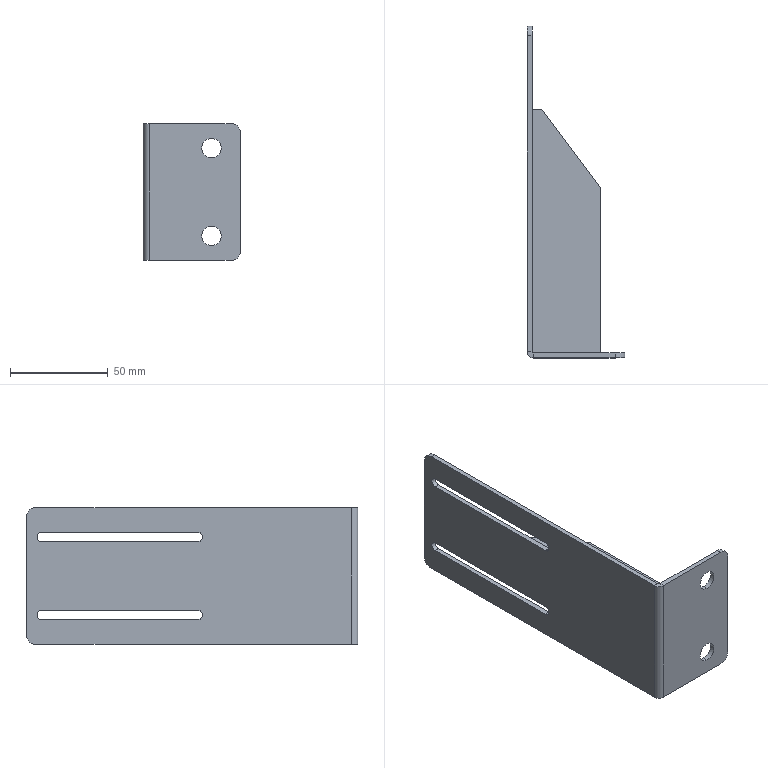Part | SolidWorks | features HoleWzd 2, BreakCorner 1, FlatPattern 1, Gusset 1, SMBaseFlange 1, SheetMetal 1 | 2 solids | 37 faces | box 50 x 170 x 70 mm | volume 44894 mm3 | plane 23 | cylinder 14 | commonest cylinder face diameters 10 x8 4.8 x4 1.473 x1 6.473 x1
STEP:
#1=CARTESIAN_POINT('',(35.,0.,7.5));
#2=VERTEX_POINT('',#1);
#3=CARTESIAN_POINT('',(35.,0.,17.5));
#4=VERTEX_POINT('',#3);
#5=CARTESIAN_POINT('',(35.,0.,12.5));
#6=DIRECTION('',(0.,1.,0.));
#7=DIRECTION('',(0.,0.,1.));
#8=AXIS2_PLACEMENT_3D('',#5,#6,#7);
#9=CIRCLE('',#8,5.);
#10=EDGE_CURVE('',#2,#4,#9,.T.);
#11=ORIENTED_EDGE('',*,*,#10,.F.);
#12=CARTESIAN_POINT('',(35.,2.5,7.5));
#13=VERTEX_POINT('',#12);
#14=CARTESIAN_POINT('',(35.,2.5,7.5));
#15=DIRECTION('',(0.,1.,0.));
#16=VECTOR('',#15,1000.);
#17=LINE('',#14,#16);
#18=EDGE_CURVE('',#2,#13,#17,.T.);
#19=ORIENTED_EDGE('',*,*,#18,.T.);
#20=CARTESIAN_POINT('',(35.,2.5,17.5));
#21=VERTEX_POINT('',#20);
#22=CARTESIAN_POINT('',(35.,2.5,12.5));
#23=DIRECTION('',(0.,1.,0.));
#24=DIRECTION('',(0.,0.,1.));
#25=AXIS2_PLACEMENT_3D('',#22,#23,#24);
#26=CIRCLE('',#25,5.);
#27=EDGE_CURVE('',#13,#21,#26,.T.);
#28=ORIENTED_EDGE('',*,*,#27,.T.);
#29=CARTESIAN_POINT('',(35.,2.5,17.5));
#30=DIRECTION('',(0.,1.,0.));
#31=VECTOR('',#30,1000.);
#32=LINE('',#29,#31);
#33=EDGE_CURVE('',#4,#21,#32,.T.);
#34=ORIENTED_EDGE('',*,*,#33,.F.);
#35=EDGE_LOOP('',(#11,#19,#28,#34));
#36=FACE_OUTER_BOUND('',#35,.T.);
#37=CARTESIAN_POINT('',(35.,2.5,12.5));
#38=DIRECTION('',(0.,1.,0.));
#39=DIRECTION('',(0.,0.,1.));
#40=AXIS2_PLACEMENT_3D('',#37,#38,#39);
#41=CYLINDRICAL_SURFACE('',#40,5.);
#42=ADVANCED_FACE('',(#36),#41,.F.);
#43=CARTESIAN_POINT('',(35.,0.,52.5));
#44=VERTEX_POINT('',#43);
#45=CARTESIAN_POINT('',(35.,0.,62.5));
#46=VERTEX_POINT('',#45);
#47=CARTESIAN_POINT('',(35.,0.,57.5));
#48=DIRECTION('',(0.,1.,0.));
#49=DIRECTION('',(0.,0.,1.));
#50=AXIS2_PLACEMENT_3D('',#47,#48,#49);
#51=CIRCLE('',#50,5.);
#52=EDGE_CURVE('',#44,#46,#51,.T.);
#53=ORIENTED_EDGE('',*,*,#52,.F.);
#54=CARTESIAN_POINT('',(35.,2.5,52.5));
#55=VERTEX_POINT('',#54);
#56=CARTESIAN_POINT('',(35.,2.5,52.5));
#57=DIRECTION('',(0.,1.,0.));
#58=VECTOR('',#57,1000.);
#59=LINE('',#56,#58);
#60=EDGE_CURVE('',#44,#55,#59,.T.);
#61=ORIENTED_EDGE('',*,*,#60,.T.);
#62=CARTESIAN_POINT('',(35.,2.5,62.5));
#63=VERTEX_POINT('',#62);
#64=CARTESIAN_POINT('',(35.,2.5,57.5));
#65=DIRECTION('',(0.,1.,0.));
#66=DIRECTION('',(0.,0.,1.));
#67=AXIS2_PLACEMENT_3D('',#64,#65,#66);
#68=CIRCLE('',#67,5.);
#69=EDGE_CURVE('',#55,#63,#68,.T.);
#70=ORIENTED_EDGE('',*,*,#69,.T.);
#71=CARTESIAN_POINT('',(35.,2.5,62.5));
#72=DIRECTION('',(0.,1.,0.));
#73=VECTOR('',#72,1000.);
#74=LINE('',#71,#73);
#75=EDGE_CURVE('',#46,#63,#74,.T.);
#76=ORIENTED_EDGE('',*,*,#75,.F.);
#77=EDGE_LOOP('',(#53,#61,#70,#76));
#78=FACE_OUTER_BOUND('',#77,.T.);
#79=CARTESIAN_POINT('',(35.,2.5,57.5));
#80=DIRECTION('',(0.,1.,0.));
#81=DIRECTION('',(0.,0.,1.));
#82=AXIS2_PLACEMENT_3D('',#79,#80,#81);
#83=CYLINDRICAL_SURFACE('',#82,5.);
#84=ADVANCED_FACE('',(#78),#83,.F.);
#85=CARTESIAN_POINT('',(35.,2.5,57.5));
#86=DIRECTION('',(0.,1.,0.));
#87=DIRECTION('',(0.,0.,1.));
#88=AXIS2_PLACEMENT_3D('',#85,#86,#87);
#89=CIRCLE('',#88,5.);
#90=EDGE_CURVE('',#63,#55,#89,.T.);
#91=ORIENTED_EDGE('',*,*,#90,.F.);
#92=ORIENTED_EDGE('',*,*,#69,.F.);
#93=EDGE_LOOP('',(#91,#92));
#94=FACE_BOUND('',#93,.T.);
#95=CARTESIAN_POINT('',(45.,2.5,70.));
#96=VERTEX_POINT('',#95);
#97=CARTESIAN_POINT('',(3.237,2.5,70.));
#98=VERTEX_POINT('',#97);
#99=CARTESIAN_POINT('',(0.,2.5,70.));
#100=DIRECTION('',(-1.,0.,0.));
#101=VECTOR('',#100,1000.);
#102=LINE('',#99,#101);
#103=EDGE_CURVE('',#96,#98,#102,.T.);
#104=ORIENTED_EDGE('',*,*,#103,.F.);
#105=CARTESIAN_POINT('',(50.,2.5,65.));
#106=VERTEX_POINT('',#105);
#107=CARTESIAN_POINT('',(45.,2.5,65.));
#108=DIRECTION('',(0.,1.,0.));
#109=DIRECTION('',(0.,0.,-1.));
#110=AXIS2_PLACEMENT_3D('',#107,#108,#109);
#111=CIRCLE('',#110,5.);
#112=EDGE_CURVE('',#96,#106,#111,.T.);
#113=ORIENTED_EDGE('',*,*,#112,.T.);
#114=CARTESIAN_POINT('',(50.,2.5,5.));
#115=VERTEX_POINT('',#114);
#116=CARTESIAN_POINT('',(50.,2.5,70.));
#117=DIRECTION('',(0.,0.,-1.));
#118=VECTOR('',#117,1000.);
#119=LINE('',#116,#118);
#120=EDGE_CURVE('',#106,#115,#119,.T.);
#121=ORIENTED_EDGE('',*,*,#120,.T.);
#122=CARTESIAN_POINT('',(45.,2.5,0.));
#123=VERTEX_POINT('',#122);
#124=CARTESIAN_POINT('',(45.,2.5,5.));
#125=DIRECTION('',(0.,1.,0.));
#126=DIRECTION('',(0.,0.,-1.));
#127=AXIS2_PLACEMENT_3D('',#124,#125,#126);
#128=CIRCLE('',#127,5.);
#129=EDGE_CURVE('',#115,#123,#128,.T.);
#130=ORIENTED_EDGE('',*,*,#129,.T.);
#131=CARTESIAN_POINT('',(3.237,2.5,0.));
#132=VERTEX_POINT('',#131);
#133=CARTESIAN_POINT('',(0.,2.5,0.));
#134=DIRECTION('',(-1.,0.,0.));
#135=VECTOR('',#134,1000.);
#136=LINE('',#133,#135);
#137=EDGE_CURVE('',#123,#132,#136,.T.);
#138=ORIENTED_EDGE('',*,*,#137,.T.);
#139=CARTESIAN_POINT('',(3.237,2.5,70.));
#140=DIRECTION('',(0.,0.,-1.));
#141=VECTOR('',#140,1000.);
#142=LINE('',#139,#141);
#143=EDGE_CURVE('',#98,#132,#142,.T.);
#144=ORIENTED_EDGE('',*,*,#143,.F.);
#145=EDGE_LOOP('',(#104,#113,#121,#130,#138,#144));
#146=FACE_OUTER_BOUND('',#145,.T.);
#147=CARTESIAN_POINT('',(35.,2.5,12.5));
#148=DIRECTION('',(0.,1.,0.));
#149=DIRECTION('',(0.,0.,1.));
#150=AXIS2_PLACEMENT_3D('',#147,#148,#149);
#151=CIRCLE('',#150,5.);
#152=EDGE_CURVE('',#21,#13,#151,.T.);
#153=ORIENTED_EDGE('',*,*,#152,.F.);
#154=ORIENTED_EDGE('',*,*,#27,.F.);
#155=EDGE_LOOP('',(#153,#154));
#156=FACE_BOUND('',#155,.T.);
#157=CARTESIAN_POINT('',(0.,2.5,70.));
#158=DIRECTION('',(0.,-1.,0.));
#159=DIRECTION('',(0.,0.,-1.));
#160=AXIS2_PLACEMENT_3D('',#157,#158,#159);
#161=PLANE('',#160);
#162=ADVANCED_FACE('',(#94,#146,#156),#161,.F.);
#163=CARTESIAN_POINT('',(0.,82.,57.4));
#164=VERTEX_POINT('',#163);
#165=CARTESIAN_POINT('',(0.,162.,57.4));
#166=VERTEX_POINT('',#165);
#167=CARTESIAN_POINT('',(0.,82.,57.4));
#168=DIRECTION('',(0.,1.,0.));
#169=VECTOR('',#168,1000.);
#170=LINE('',#167,#169);
#171=EDGE_CURVE('',#164,#166,#170,.T.);
#172=ORIENTED_EDGE('',*,*,#171,.F.);
#173=CARTESIAN_POINT('',(0.,82.,52.6));
#174=VERTEX_POINT('',#173);
#175=CARTESIAN_POINT('',(0.,82.,55.));
#176=DIRECTION('',(1.,0.,0.));
#177=DIRECTION('',(0.,0.,-1.));
#178=AXIS2_PLACEMENT_3D('',#175,#176,#177);
#179=CIRCLE('',#178,2.4);
#180=EDGE_CURVE('',#164,#174,#179,.T.);
#181=ORIENTED_EDGE('',*,*,#180,.T.);
#182=CARTESIAN_POINT('',(0.,162.,52.6));
#183=VERTEX_POINT('',#182);
#184=CARTESIAN_POINT('',(0.,82.,52.6));
#185=DIRECTION('',(0.,1.,0.));
#186=VECTOR('',#185,1000.);
#187=LINE('',#184,#186);
#188=EDGE_CURVE('',#174,#183,#187,.T.);
#189=ORIENTED_EDGE('',*,*,#188,.T.);
#190=CARTESIAN_POINT('',(0.,162.,55.));
#191=DIRECTION('',(1.,0.,0.));
#192=DIRECTION('',(0.,0.,-1.));
#193=AXIS2_PLACEMENT_3D('',#190,#191,#192);
#194=CIRCLE('',#193,2.4);
#195=EDGE_CURVE('',#183,#166,#194,.T.);
#196=ORIENTED_EDGE('',*,*,#195,.T.);
#197=EDGE_LOOP('',(#172,#181,#189,#196));
#198=FACE_BOUND('',#197,.T.);
#199=CARTESIAN_POINT('',(0.,3.237,70.));
#200=VERTEX_POINT('',#199);
#201=CARTESIAN_POINT('',(0.,165.,70.));
#202=VERTEX_POINT('',#201);
#203=CARTESIAN_POINT('',(0.,0.,70.));
#204=DIRECTION('',(0.,1.,0.));
#205=VECTOR('',#204,1000.);
#206=LINE('',#203,#205);
#207=EDGE_CURVE('',#200,#202,#206,.T.);
#208=ORIENTED_EDGE('',*,*,#207,.T.);
#209=CARTESIAN_POINT('',(0.,170.,65.));
#210=VERTEX_POINT('',#209);
#211=CARTESIAN_POINT('',(0.,165.,65.));
#212=DIRECTION('',(-1.,0.,0.));
#213=DIRECTION('',(0.,0.,1.));
#214=AXIS2_PLACEMENT_3D('',#211,#212,#213);
#215=CIRCLE('',#214,5.);
#216=EDGE_CURVE('',#202,#210,#215,.T.);
#217=ORIENTED_EDGE('',*,*,#216,.T.);
#218=CARTESIAN_POINT('',(0.,170.,5.));
#219=VERTEX_POINT('',#218);
#220=CARTESIAN_POINT('',(0.,170.,70.));
#221=DIRECTION('',(0.,0.,-1.));
#222=VECTOR('',#221,1000.);
#223=LINE('',#220,#222);
#224=EDGE_CURVE('',#210,#219,#223,.T.);
#225=ORIENTED_EDGE('',*,*,#224,.T.);
#226=CARTESIAN_POINT('',(0.,165.,0.));
#227=VERTEX_POINT('',#226);
#228=CARTESIAN_POINT('',(0.,165.,5.));
#229=DIRECTION('',(-1.,0.,0.));
#230=DIRECTION('',(0.,0.,1.));
#231=AXIS2_PLACEMENT_3D('',#228,#229,#230);
#232=CIRCLE('',#231,5.);
#233=EDGE_CURVE('',#219,#227,#232,.T.);
#234=ORIENTED_EDGE('',*,*,#233,.T.);
#235=CARTESIAN_POINT('',(0.,3.237,0.));
#236=VERTEX_POINT('',#235);
#237=CARTESIAN_POINT('',(0.,0.,0.));
#238=DIRECTION('',(0.,1.,0.));
#239=VECTOR('',#238,1000.);
#240=LINE('',#237,#239);
#241=EDGE_CURVE('',#236,#227,#240,.T.);
#242=ORIENTED_EDGE('',*,*,#241,.F.);
#243=CARTESIAN_POINT('',(0.,3.237,70.));
#244=DIRECTION('',(0.,0.,-1.));
#245=VECTOR('',#244,1000.);
#246=LINE('',#243,#245);
#247=EDGE_CURVE('',#200,#236,#246,.T.);
#248=ORIENTED_EDGE('',*,*,#247,.F.);
#249=EDGE_LOOP('',(#208,#217,#225,#234,#242,#248));
#250=FACE_OUTER_BOUND('',#249,.T.);
#251=CARTESIAN_POINT('',(0.,82.,17.4));
#252=VERTEX_POINT('',#251);
#253=CARTESIAN_POINT('',(0.,82.,12.6));
#254=VERTEX_POINT('',#253);
#255=CARTESIAN_POINT('',(0.,82.,15.));
#256=DIRECTION('',(1.,0.,0.));
#257=DIRECTION('',(0.,0.,-1.));
#258=AXIS2_PLACEMENT_3D('',#255,#256,#257);
#259=CIRCLE('',#258,2.4);
#260=EDGE_CURVE('',#252,#254,#259,.T.);
#261=ORIENTED_EDGE('',*,*,#260,.T.);
#262=CARTESIAN_POINT('',(0.,162.,12.6));
#263=VERTEX_POINT('',#262);
#264=CARTESIAN_POINT('',(0.,82.,12.6));
#265=DIRECTION('',(0.,1.,0.));
#266=VECTOR('',#265,1000.);
#267=LINE('',#264,#266);
#268=EDGE_CURVE('',#254,#263,#267,.T.);
#269=ORIENTED_EDGE('',*,*,#268,.T.);
#270=CARTESIAN_POINT('',(0.,162.,17.4));
#271=VERTEX_POINT('',#270);
#272=CARTESIAN_POINT('',(0.,162.,15.));
#273=DIRECTION('',(1.,0.,0.));
#274=DIRECTION('',(0.,0.,-1.));
#275=AXIS2_PLACEMENT_3D('',#272,#273,#274);
#276=CIRCLE('',#275,2.4);
#277=EDGE_CURVE('',#263,#271,#276,.T.);
#278=ORIENTED_EDGE('',*,*,#277,.T.);
#279=CARTESIAN_POINT('',(0.,82.,17.4));
#280=DIRECTION('',(0.,1.,0.));
#281=VECTOR('',#280,1000.);
#282=LINE('',#279,#281);
#283=EDGE_CURVE('',#252,#271,#282,.T.);
#284=ORIENTED_EDGE('',*,*,#283,.F.);
#285=EDGE_LOOP('',(#261,#269,#278,#284));
#286=FACE_BOUND('',#285,.T.);
#287=CARTESIAN_POINT('',(0.,0.,70.));
#288=DIRECTION('',(-1.,0.,0.));
#289=DIRECTION('',(0.,0.,1.));
#290=AXIS2_PLACEMENT_3D('',#287,#288,#289);
#291=PLANE('',#290);
#292=ADVANCED_FACE('',(#198,#250,#286),#291,.T.);
#293=CARTESIAN_POINT('',(2.5,3.237,70.));
#294=VERTEX_POINT('',#293);
#295=CARTESIAN_POINT('',(0.,3.237,70.));
#296=DIRECTION('',(1.,0.,0.));
#297=VECTOR('',#296,1000.);
#298=LINE('',#295,#297);
#299=EDGE_CURVE('',#200,#294,#298,.T.);
#300=ORIENTED_EDGE('',*,*,#299,.F.);
#301=CARTESIAN_POINT('',(3.237,0.,70.));
#302=VERTEX_POINT('',#301);
#303=CARTESIAN_POINT('',(3.237,3.237,70.));
#304=DIRECTION('',(0.,0.,-1.));
#305=DIRECTION('',(1.,0.,0.));
#306=AXIS2_PLACEMENT_3D('',#303,#304,#305);
#307=CIRCLE('',#306,3.237);
#308=EDGE_CURVE('',#302,#200,#307,.T.);
#309=ORIENTED_EDGE('',*,*,#308,.F.);
#310=CARTESIAN_POINT('',(3.237,2.5,70.));
#311=DIRECTION('',(0.,-1.,0.));
#312=VECTOR('',#311,1000.);
#313=LINE('',#310,#312);
#314=EDGE_CURVE('',#98,#302,#313,.T.);
#315=ORIENTED_EDGE('',*,*,#314,.F.);
#316=CARTESIAN_POINT('',(3.237,3.237,70.));
#317=DIRECTION('',(0.,0.,-1.));
#318=DIRECTION('',(1.,0.,0.));
#319=AXIS2_PLACEMENT_3D('',#316,#317,#318);
#320=CIRCLE('',#319,0.7366);
#321=EDGE_CURVE('',#98,#294,#320,.T.);
#322=ORIENTED_EDGE('',*,*,#321,.T.);
#323=EDGE_LOOP('',(#300,#309,#315,#322));
#324=FACE_OUTER_BOUND('',#323,.T.);
#325=CARTESIAN_POINT('',(0.,3.237,70.));
#326=DIRECTION('',(0.,0.,1.));
#327=DIRECTION('',(1.,0.,0.));
#328=AXIS2_PLACEMENT_3D('',#325,#326,#327);
#329=PLANE('',#328);
#330=ADVANCED_FACE('',(#324),#329,.T.);
#331=CARTESIAN_POINT('',(2.5,165.,70.));
#332=VERTEX_POINT('',#331);
#333=CARTESIAN_POINT('',(2.5,0.,70.));
#334=DIRECTION('',(0.,1.,0.));
#335=VECTOR('',#334,1000.);
#336=LINE('',#333,#335);
#337=EDGE_CURVE('',#294,#332,#336,.T.);
#338=ORIENTED_EDGE('',*,*,#337,.T.);
#339=CARTESIAN_POINT('',(3.237,165.,70.));
#340=DIRECTION('',(-1.,0.,0.));
#341=VECTOR('',#340,1000.);
#342=LINE('',#339,#341);
#343=EDGE_CURVE('',#332,#202,#342,.T.);
#344=ORIENTED_EDGE('',*,*,#343,.T.);
#345=ORIENTED_EDGE('',*,*,#207,.F.);
#346=ORIENTED_EDGE('',*,*,#299,.T.);
#347=EDGE_LOOP('',(#338,#344,#345,#346));
#348=FACE_OUTER_BOUND('',#347,.T.);
#349=CARTESIAN_POINT('',(3.237,2.5,70.));
#350=DIRECTION('',(0.,0.,1.));
#351=DIRECTION('',(1.,0.,0.));
#352=AXIS2_PLACEMENT_3D('',#349,#350,#351);
#353=PLANE('',#352);
#354=ADVANCED_FACE('',(#348),#353,.T.);
#355=CARTESIAN_POINT('',(3.237,0.,0.));
#356=VERTEX_POINT('',#355);
#357=CARTESIAN_POINT('',(3.237,0.,0.));
#358=DIRECTION('',(0.,1.,0.));
#359=VECTOR('',#358,1000.);
#360=LINE('',#357,#359);
#361=EDGE_CURVE('',#356,#132,#360,.T.);
#362=ORIENTED_EDGE('',*,*,#361,.F.);
#363=CARTESIAN_POINT('',(3.237,3.237,0.));
#364=DIRECTION('',(0.,0.,-1.));
#365=DIRECTION('',(1.,0.,0.));
#366=AXIS2_PLACEMENT_3D('',#363,#364,#365);
#367=CIRCLE('',#366,3.237);
#368=EDGE_CURVE('',#356,#236,#367,.T.);
#369=ORIENTED_EDGE('',*,*,#368,.T.);
#370=CARTESIAN_POINT('',(2.5,3.237,0.));
#371=VERTEX_POINT('',#370);
#372=CARTESIAN_POINT('',(2.5,3.237,0.));
#373=DIRECTION('',(-1.,0.,0.));
#374=VECTOR('',#373,1000.);
#375=LINE('',#372,#374);
#376=EDGE_CURVE('',#371,#236,#375,.T.);
#377=ORIENTED_EDGE('',*,*,#376,.F.);
#378=CARTESIAN_POINT('',(3.237,3.237,0.));
#379=DIRECTION('',(0.,0.,-1.));
#380=DIRECTION('',(1.,0.,0.));
#381=AXIS2_PLACEMENT_3D('',#378,#379,#380);
#382=CIRCLE('',#381,0.7366);
#383=EDGE_CURVE('',#132,#371,#382,.T.);
#384=ORIENTED_EDGE('',*,*,#383,.F.);
#385=EDGE_LOOP('',(#362,#369,#377,#384));
#386=FACE_OUTER_BOUND('',#385,.T.);
#387=CARTESIAN_POINT('',(3.237,0.,0.));
#388=DIRECTION('',(0.,0.,-1.));
#389=DIRECTION('',(-1.,0.,0.));
#390=AXIS2_PLACEMENT_3D('',#387,#388,#389);
#391=PLANE('',#390);
#392=ADVANCED_FACE('',(#386),#391,.T.);
#393=ORIENTED_EDGE('',*,*,#137,.F.);
#394=CARTESIAN_POINT('',(45.,0.,0.));
#395=VERTEX_POINT('',#394);
#396=CARTESIAN_POINT('',(45.,3.237,0.));
#397=DIRECTION('',(0.,-1.,0.));
#398=VECTOR('',#397,1000.);
#399=LINE('',#396,#398);
#400=EDGE_CURVE('',#123,#395,#399,.T.);
#401=ORIENTED_EDGE('',*,*,#400,.T.);
#402=CARTESIAN_POINT('',(0.,0.,0.));
#403=DIRECTION('',(-1.,0.,0.));
#404=VECTOR('',#403,1000.);
#405=LINE('',#402,#404);
#406=EDGE_CURVE('',#395,#356,#405,.T.);
#407=ORIENTED_EDGE('',*,*,#406,.T.);
#408=ORIENTED_EDGE('',*,*,#361,.T.);
#409=EDGE_LOOP('',(#393,#401,#407,#408));
#410=FACE_OUTER_BOUND('',#409,.T.);
#411=CARTESIAN_POINT('',(2.5,3.237,0.));
#412=DIRECTION('',(0.,0.,-1.));
#413=DIRECTION('',(-1.,0.,0.));
#414=AXIS2_PLACEMENT_3D('',#411,#412,#413);
#415=PLANE('',#414);
#416=ADVANCED_FACE('',(#410),#415,.T.);
#417=CARTESIAN_POINT('',(2.5,82.,57.4));
#418=VERTEX_POINT('',#417);
#419=CARTESIAN_POINT('',(2.5,82.,52.6));
#420=VERTEX_POINT('',#419);
#421=CARTESIAN_POINT('',(2.5,82.,55.));
#422=DIRECTION('',(1.,0.,0.));
#423=DIRECTION('',(0.,0.,-1.));
#424=AXIS2_PLACEMENT_3D('',#421,#422,#423);
#425=CIRCLE('',#424,2.4);
#426=EDGE_CURVE('',#418,#420,#425,.T.);
#427=ORIENTED_EDGE('',*,*,#426,.F.);
#428=CARTESIAN_POINT('',(2.5,162.,57.4));
#429=VERTEX_POINT('',#428);
#430=CARTESIAN_POINT('',(2.5,82.,57.4));
#431=DIRECTION('',(0.,1.,0.));
#432=VECTOR('',#431,1000.);
#433=LINE('',#430,#432);
#434=EDGE_CURVE('',#418,#429,#433,.T.);
#435=ORIENTED_EDGE('',*,*,#434,.T.);
#436=CARTESIAN_POINT('',(2.5,162.,52.6));
#437=VERTEX_POINT('',#436);
#438=CARTESIAN_POINT('',(2.5,162.,55.));
#439=DIRECTION('',(1.,0.,0.));
#440=DIRECTION('',(0.,0.,-1.));
#441=AXIS2_PLACEMENT_3D('',#438,#439,#440);
#442=CIRCLE('',#441,2.4);
#443=EDGE_CURVE('',#437,#429,#442,.T.);
#444=ORIENTED_EDGE('',*,*,#443,.F.);
#445=CARTESIAN_POINT('',(2.5,82.,52.6));
#446=DIRECTION('',(0.,1.,0.));
#447=VECTOR('',#446,1000.);
#448=LINE('',#445,#447);
#449=EDGE_CURVE('',#420,#437,#448,.T.);
#450=ORIENTED_EDGE('',*,*,#449,.F.);
#451=EDGE_LOOP('',(#427,#435,#444,#450));
#452=FACE_BOUND('',#451,.T.);
#453=CARTESIAN_POINT('',(2.5,82.,17.4));
#454=VERTEX_POINT('',#453);
#455=CARTESIAN_POINT('',(2.5,162.,17.4));
#456=VERTEX_POINT('',#455);
#457=CARTESIAN_POINT('',(2.5,82.,17.4));
#458=DIRECTION('',(0.,1.,0.));
#459=VECTOR('',#458,1000.);
#460=LINE('',#457,#459);
#461=EDGE_CURVE('',#454,#456,#460,.T.);
#462=ORIENTED_EDGE('',*,*,#461,.T.);
#463=CARTESIAN_POINT('',(2.5,162.,12.6));
#464=VERTEX_POINT('',#463);
#465=CARTESIAN_POINT('',(2.5,162.,15.));
#466=DIRECTION('',(1.,0.,0.));
#467=DIRECTION('',(0.,0.,-1.));
#468=AXIS2_PLACEMENT_3D('',#465,#466,#467);
#469=CIRCLE('',#468,2.4);
#470=EDGE_CURVE('',#464,#456,#469,.T.);
#471=ORIENTED_EDGE('',*,*,#470,.F.);
#472=CARTESIAN_POINT('',(2.5,82.,12.6));
#473=VERTEX_POINT('',#472);
#474=CARTESIAN_POINT('',(2.5,82.,12.6));
#475=DIRECTION('',(0.,1.,0.));
#476=VECTOR('',#475,1000.);
#477=LINE('',#474,#476);
#478=EDGE_CURVE('',#473,#464,#477,.T.);
#479=ORIENTED_EDGE('',*,*,#478,.F.);
#480=CARTESIAN_POINT('',(2.5,82.,15.));
#481=DIRECTION('',(1.,0.,0.));
#482=DIRECTION('',(0.,0.,-1.));
#483=AXIS2_PLACEMENT_3D('',#480,#481,#482);
#484=CIRCLE('',#483,2.4);
#485=EDGE_CURVE('',#454,#473,#484,.T.);
#486=ORIENTED_EDGE('',*,*,#485,.F.);
#487=EDGE_LOOP('',(#462,#471,#479,#486));
#488=FACE_BOUND('',#487,.T.);
#489=CARTESIAN_POINT('',(2.5,170.,65.));
#490=VERTEX_POINT('',#489);
#491=CARTESIAN_POINT('',(2.5,170.,5.));
#492=VERTEX_POINT('',#491);
#493=CARTESIAN_POINT('',(2.5,170.,70.));
#494=DIRECTION('',(0.,0.,-1.));
#495=VECTOR('',#494,1000.);
#496=LINE('',#493,#495);
#497=EDGE_CURVE('',#490,#492,#496,.T.);
#498=ORIENTED_EDGE('',*,*,#497,.F.);
#499=CARTESIAN_POINT('',(2.5,165.,65.));
#500=DIRECTION('',(1.,0.,0.));
#501=DIRECTION('',(0.,0.,1.));
#502=AXIS2_PLACEMENT_3D('',#499,#500,#501);
#503=CIRCLE('',#502,5.);
#504=EDGE_CURVE('',#490,#332,#503,.T.);
#505=ORIENTED_EDGE('',*,*,#504,.T.);
#506=ORIENTED_EDGE('',*,*,#337,.F.);
#507=CARTESIAN_POINT('',(2.5,3.237,70.));
#508=DIRECTION('',(0.,0.,-1.));
#509=VECTOR('',#508,1000.);
#510=LINE('',#507,#509);
#511=EDGE_CURVE('',#294,#371,#510,.T.);
#512=ORIENTED_EDGE('',*,*,#511,.T.);
#513=CARTESIAN_POINT('',(2.5,165.,0.));
#514=VERTEX_POINT('',#513);
#515=CARTESIAN_POINT('',(2.5,0.,0.));
#516=DIRECTION('',(0.,1.,0.));
#517=VECTOR('',#516,1000.);
#518=LINE('',#515,#517);
#519=EDGE_CURVE('',#371,#514,#518,.T.);
#520=ORIENTED_EDGE('',*,*,#519,.T.);
#521=CARTESIAN_POINT('',(2.5,165.,5.));
#522=DIRECTION('',(1.,0.,0.));
#523=DIRECTION('',(0.,0.,1.));
#524=AXIS2_PLACEMENT_3D('',#521,#522,#523);
#525=CIRCLE('',#524,5.);
#526=EDGE_CURVE('',#514,#492,#525,.T.);
#527=ORIENTED_EDGE('',*,*,#526,.T.);
#528=EDGE_LOOP('',(#498,#505,#506,#512,#520,#527));
#529=FACE_OUTER_BOUND('',#528,.T.);
#530=CARTESIAN_POINT('',(2.5,0.,70.));
#531=DIRECTION('',(-1.,0.,0.));
#532=DIRECTION('',(0.,0.,1.));
#533=AXIS2_PLACEMENT_3D('',#530,#531,#532);
#534=PLANE('',#533);
#535=ADVANCED_FACE('',(#452,#488,#529),#534,.F.);
#536=ORIENTED_EDGE('',*,*,#224,.F.);
#537=CARTESIAN_POINT('',(0.,170.,65.));
#538=DIRECTION('',(1.,0.,0.));
#539=VECTOR('',#538,1000.);
#540=LINE('',#537,#539);
#541=EDGE_CURVE('',#210,#490,#540,.T.);
#542=ORIENTED_EDGE('',*,*,#541,.T.);
#543=ORIENTED_EDGE('',*,*,#497,.T.);
#544=CARTESIAN_POINT('',(0.,170.,5.));
#545=DIRECTION('',(-1.,0.,0.));
#546=VECTOR('',#545,1000.);
#547=LINE('',#544,#546);
#548=EDGE_CURVE('',#492,#219,#547,.T.);
#549=ORIENTED_EDGE('',*,*,#548,.T.);
#550=EDGE_LOOP('',(#536,#542,#543,#549));
#551=FACE_OUTER_BOUND('',#550,.T.);
#552=CARTESIAN_POINT('',(0.,170.,70.));
#553=DIRECTION('',(0.,1.,0.));
#554=DIRECTION('',(0.,0.,1.));
#555=AXIS2_PLACEMENT_3D('',#552,#553,#554);
#556=PLANE('',#555);
#557=ADVANCED_FACE('',(#551),#556,.T.);
#558=ORIENTED_EDGE('',*,*,#368,.F.);
#559=CARTESIAN_POINT('',(3.237,0.,70.));
#560=DIRECTION('',(0.,0.,-1.));
#561=VECTOR('',#560,1000.);
#562=LINE('',#559,#561);
#563=EDGE_CURVE('',#302,#356,#562,.T.);
#564=ORIENTED_EDGE('',*,*,#563,.F.);
#565=ORIENTED_EDGE('',*,*,#308,.T.);
#566=ORIENTED_EDGE('',*,*,#247,.T.);
#567=EDGE_LOOP('',(#558,#564,#565,#566));
#568=FACE_OUTER_BOUND('',#567,.T.);
#569=CARTESIAN_POINT('',(3.237,3.237,70.));
#570=DIRECTION('',(0.,0.,-1.));
#571=DIRECTION('',(-1.,0.,0.));
#572=AXIS2_PLACEMENT_3D('',#569,#570,#571);
#573=CYLINDRICAL_SURFACE('',#572,3.237);
#574=ADVANCED_FACE('',(#568),#573,.T.);
#575=CARTESIAN_POINT('',(35.,0.,12.5));
#576=DIRECTION('',(0.,1.,0.));
#577=DIRECTION('',(0.,0.,1.));
#578=AXIS2_PLACEMENT_3D('',#575,#576,#577);
#579=CIRCLE('',#578,5.);
#580=EDGE_CURVE('',#4,#2,#579,.T.);
#581=ORIENTED_EDGE('',*,*,#580,.T.);
#582=ORIENTED_EDGE('',*,*,#10,.T.);
#583=EDGE_LOOP('',(#581,#582));
#584=FACE_BOUND('',#583,.T.);
#585=CARTESIAN_POINT('',(35.,0.,57.5));
#586=DIRECTION('',(0.,1.,0.));
#587=DIRECTION('',(0.,0.,1.));
#588=AXIS2_PLACEMENT_3D('',#585,#586,#587);
#589=CIRCLE('',#588,5.);
#590=EDGE_CURVE('',#46,#44,#589,.T.);
#591=ORIENTED_EDGE('',*,*,#590,.T.);
#592=ORIENTED_EDGE('',*,*,#52,.T.);
#593=EDGE_LOOP('',(#591,#592));
#594=FACE_BOUND('',#593,.T.);
#595=CARTESIAN_POINT('',(50.,0.,65.));
#596=VERTEX_POINT('',#595);
#597=CARTESIAN_POINT('',(50.,0.,5.));
#598=VERTEX_POINT('',#597);
#599=CARTESIAN_POINT('',(50.,0.,70.));
#600=DIRECTION('',(0.,0.,-1.));
#601=VECTOR('',#600,1000.);
#602=LINE('',#599,#601);
#603=EDGE_CURVE('',#596,#598,#602,.T.);
#604=ORIENTED_EDGE('',*,*,#603,.F.);
#605=CARTESIAN_POINT('',(45.,0.,70.));
#606=VERTEX_POINT('',#605);
#607=CARTESIAN_POINT('',(45.,0.,65.));
#608=DIRECTION('',(0.,-1.,0.));
#609=DIRECTION('',(0.,0.,-1.));
#610=AXIS2_PLACEMENT_3D('',#607,#608,#609);
#611=CIRCLE('',#610,5.);
#612=EDGE_CURVE('',#596,#606,#611,.T.);
#613=ORIENTED_EDGE('',*,*,#612,.T.);
#614=CARTESIAN_POINT('',(0.,0.,70.));
#615=DIRECTION('',(-1.,0.,0.));
#616=VECTOR('',#615,1000.);
#617=LINE('',#614,#616);
#618=EDGE_CURVE('',#606,#302,#617,.T.);
#619=ORIENTED_EDGE('',*,*,#618,.T.);
#620=ORIENTED_EDGE('',*,*,#563,.T.);
#621=ORIENTED_EDGE('',*,*,#406,.F.);
#622=CARTESIAN_POINT('',(45.,0.,5.));
#623=DIRECTION('',(0.,-1.,0.));
#624=DIRECTION('',(0.,0.,-1.));
#625=AXIS2_PLACEMENT_3D('',#622,#623,#624);
#626=CIRCLE('',#625,5.);
#627=EDGE_CURVE('',#395,#598,#626,.T.);
#628=ORIENTED_EDGE('',*,*,#627,.T.);
#629=EDGE_LOOP('',(#604,#613,#619,#620,#621,#628));
#630=FACE_OUTER_BOUND('',#629,.T.);
#631=CARTESIAN_POINT('',(0.,0.,70.));
#632=DIRECTION('',(0.,-1.,0.));
#633=DIRECTION('',(0.,0.,-1.));
#634=AXIS2_PLACEMENT_3D('',#631,#632,#633);
#635=PLANE('',#634);
#636=ADVANCED_FACE('',(#584,#594,#630),#635,.T.);
#637=ORIENTED_EDGE('',*,*,#120,.F.);
#638=CARTESIAN_POINT('',(50.,2.5,65.));
#639=DIRECTION('',(0.,-1.,0.));
#640=VECTOR('',#639,1000.);
#641=LINE('',#638,#640);
#642=EDGE_CURVE('',#106,#596,#641,.T.);
#643=ORIENTED_EDGE('',*,*,#642,.T.);
#644=ORIENTED_EDGE('',*,*,#603,.T.);
#645=CARTESIAN_POINT('',(50.,2.5,5.));
#646=DIRECTION('',(0.,1.,0.));
#647=VECTOR('',#646,1000.);
#648=LINE('',#645,#647);
#649=EDGE_CURVE('',#598,#115,#648,.T.);
#650=ORIENTED_EDGE('',*,*,#649,.T.);
#651=EDGE_LOOP('',(#637,#643,#644,#650));
#652=FACE_OUTER_BOUND('',#651,.T.);
#653=CARTESIAN_POINT('',(50.,2.5,70.));
#654=DIRECTION('',(1.,0.,0.));
#655=DIRECTION('',(0.,0.,-1.));
#656=AXIS2_PLACEMENT_3D('',#653,#654,#655);
#657=PLANE('',#656);
#658=ADVANCED_FACE('',(#652),#657,.T.);
#659=ORIENTED_EDGE('',*,*,#383,.T.);
#660=ORIENTED_EDGE('',*,*,#511,.F.);
#661=ORIENTED_EDGE('',*,*,#321,.F.);
#662=ORIENTED_EDGE('',*,*,#143,.T.);
#663=EDGE_LOOP('',(#659,#660,#661,#662));
#664=FACE_OUTER_BOUND('',#663,.T.);
#665=CARTESIAN_POINT('',(3.237,3.237,70.));
#666=DIRECTION('',(0.,0.,-1.));
#667=DIRECTION('',(-1.,0.,0.));
#668=AXIS2_PLACEMENT_3D('',#665,#666,#667);
#669=CYLINDRICAL_SURFACE('',#668,0.7366);
#670=ADVANCED_FACE('',(#664),#669,.F.);
#671=ORIENTED_EDGE('',*,*,#618,.F.);
#672=CARTESIAN_POINT('',(45.,3.237,70.));
#673=DIRECTION('',(0.,1.,0.));
#674=VECTOR('',#673,1000.);
#675=LINE('',#672,#674);
#676=EDGE_CURVE('',#606,#96,#675,.T.);
#677=ORIENTED_EDGE('',*,*,#676,.T.);
#678=ORIENTED_EDGE('',*,*,#103,.T.);
#679=ORIENTED_EDGE('',*,*,#314,.T.);
#680=EDGE_LOOP('',(#671,#677,#678,#679));
#681=FACE_OUTER_BOUND('',#680,.T.);
#682=CARTESIAN_POINT('',(3.237,3.237,70.));
#683=DIRECTION('',(0.,0.,1.));
#684=DIRECTION('',(1.,0.,0.));
#685=AXIS2_PLACEMENT_3D('',#682,#683,#684);
#686=PLANE('',#685);
#687=ADVANCED_FACE('',(#681),#686,.T.);
#688=ORIENTED_EDGE('',*,*,#241,.T.);
#689=CARTESIAN_POINT('',(2.5,165.,0.));
#690=DIRECTION('',(1.,0.,0.));
#691=VECTOR('',#690,1000.);
#692=LINE('',#689,#691);
#693=EDGE_CURVE('',#227,#514,#692,.T.);
#694=ORIENTED_EDGE('',*,*,#693,.T.);
#695=ORIENTED_EDGE('',*,*,#519,.F.);
#696=ORIENTED_EDGE('',*,*,#376,.T.);
#697=EDGE_LOOP('',(#688,#694,#695,#696));
#698=FACE_OUTER_BOUND('',#697,.T.);
#699=CARTESIAN_POINT('',(3.237,3.237,0.));
#700=DIRECTION('',(0.,0.,1.));
#701=DIRECTION('',(1.,0.,0.));
#702=AXIS2_PLACEMENT_3D('',#699,#700,#701);
#703=PLANE('',#702);
#704=ADVANCED_FACE('',(#698),#703,.F.);
#705=ORIENTED_EDGE('',*,*,#277,.F.);
#706=CARTESIAN_POINT('',(2.5,162.,12.6));
#707=DIRECTION('',(-1.,0.,0.));
#708=VECTOR('',#707,1000.);
#709=LINE('',#706,#708);
#710=EDGE_CURVE('',#464,#263,#709,.T.);
#711=ORIENTED_EDGE('',*,*,#710,.F.);
#712=ORIENTED_EDGE('',*,*,#470,.T.);
#713=CARTESIAN_POINT('',(2.5,162.,17.4));
#714=DIRECTION('',(1.,0.,0.));
#715=VECTOR('',#714,1000.);
#716=LINE('',#713,#715);
#717=EDGE_CURVE('',#271,#456,#716,.T.);
#718=ORIENTED_EDGE('',*,*,#717,.F.);
#719=EDGE_LOOP('',(#705,#711,#712,#718));
#720=FACE_OUTER_BOUND('',#719,.T.);
#721=CARTESIAN_POINT('',(2.5,162.,15.));
#722=DIRECTION('',(1.,0.,0.));
#723=DIRECTION('',(0.,0.,-1.));
#724=AXIS2_PLACEMENT_3D('',#721,#722,#723);
#725=CYLINDRICAL_SURFACE('',#724,2.4);
#726=ADVANCED_FACE('',(#720),#725,.F.);
#727=ORIENTED_EDGE('',*,*,#485,.T.);
#728=CARTESIAN_POINT('',(2.5,82.,12.6));
#729=DIRECTION('',(1.,0.,0.));
#730=VECTOR('',#729,1000.);
#731=LINE('',#728,#730);
#732=EDGE_CURVE('',#254,#473,#731,.T.);
#733=ORIENTED_EDGE('',*,*,#732,.F.);
#734=ORIENTED_EDGE('',*,*,#260,.F.);
#735=CARTESIAN_POINT('',(2.5,82.,17.4));
#736=DIRECTION('',(-1.,0.,0.));
#737=VECTOR('',#736,1000.);
#738=LINE('',#735,#737);
#739=EDGE_CURVE('',#454,#252,#738,.T.);
#740=ORIENTED_EDGE('',*,*,#739,.F.);
#741=EDGE_LOOP('',(#727,#733,#734,#740));
#742=FACE_OUTER_BOUND('',#741,.T.);
#743=CARTESIAN_POINT('',(2.5,82.,15.));
#744=DIRECTION('',(1.,0.,0.));
#745=DIRECTION('',(0.,0.,-1.));
#746=AXIS2_PLACEMENT_3D('',#743,#744,#745);
#747=CYLINDRICAL_SURFACE('',#746,2.4);
#748=ADVANCED_FACE('',(#742),#747,.F.);
#749=ORIENTED_EDGE('',*,*,#717,.T.);
#750=ORIENTED_EDGE('',*,*,#461,.F.);
#751=ORIENTED_EDGE('',*,*,#739,.T.);
#752=ORIENTED_EDGE('',*,*,#283,.T.);
#753=EDGE_LOOP('',(#749,#750,#751,#752));
#754=FACE_OUTER_BOUND('',#753,.T.);
#755=CARTESIAN_POINT('',(2.5,82.,17.4));
#756=DIRECTION('',(0.,0.,1.));
#757=DIRECTION('',(1.,0.,0.));
#758=AXIS2_PLACEMENT_3D('',#755,#756,#757);
#759=PLANE('',#758);
#760=ADVANCED_FACE('',(#754),#759,.F.);
#761=ORIENTED_EDGE('',*,*,#710,.T.);
#762=ORIENTED_EDGE('',*,*,#268,.F.);
#763=ORIENTED_EDGE('',*,*,#732,.T.);
#764=ORIENTED_EDGE('',*,*,#478,.T.);
#765=EDGE_LOOP('',(#761,#762,#763,#764));
#766=FACE_OUTER_BOUND('',#765,.T.);
#767=CARTESIAN_POINT('',(2.5,82.,12.6));
#768=DIRECTION('',(0.,0.,-1.));
#769=DIRECTION('',(-1.,0.,0.));
#770=AXIS2_PLACEMENT_3D('',#767,#768,#769);
#771=PLANE('',#770);
#772=ADVANCED_FACE('',(#766),#771,.F.);
#773=ORIENTED_EDGE('',*,*,#195,.F.);
#774=CARTESIAN_POINT('',(2.5,162.,52.6));
#775=DIRECTION('',(-1.,0.,0.));
#776=VECTOR('',#775,1000.);
#777=LINE('',#774,#776);
#778=EDGE_CURVE('',#437,#183,#777,.T.);
#779=ORIENTED_EDGE('',*,*,#778,.F.);
#780=ORIENTED_EDGE('',*,*,#443,.T.);
#781=CARTESIAN_POINT('',(2.5,162.,57.4));
#782=DIRECTION('',(1.,0.,0.));
#783=VECTOR('',#782,1000.);
#784=LINE('',#781,#783);
#785=EDGE_CURVE('',#166,#429,#784,.T.);
#786=ORIENTED_EDGE('',*,*,#785,.F.);
#787=EDGE_LOOP('',(#773,#779,#780,#786));
#788=FACE_OUTER_BOUND('',#787,.T.);
#789=CARTESIAN_POINT('',(2.5,162.,55.));
#790=DIRECTION('',(1.,0.,0.));
#791=DIRECTION('',(0.,0.,-1.));
#792=AXIS2_PLACEMENT_3D('',#789,#790,#791);
#793=CYLINDRICAL_SURFACE('',#792,2.4);
#794=ADVANCED_FACE('',(#788),#793,.F.);
#795=ORIENTED_EDGE('',*,*,#426,.T.);
#796=CARTESIAN_POINT('',(2.5,82.,52.6));
#797=DIRECTION('',(1.,0.,0.));
#798=VECTOR('',#797,1000.);
#799=LINE('',#796,#798);
#800=EDGE_CURVE('',#174,#420,#799,.T.);
#801=ORIENTED_EDGE('',*,*,#800,.F.);
#802=ORIENTED_EDGE('',*,*,#180,.F.);
#803=CARTESIAN_POINT('',(2.5,82.,57.4));
#804=DIRECTION('',(-1.,0.,0.));
#805=VECTOR('',#804,1000.);
#806=LINE('',#803,#805);
#807=EDGE_CURVE('',#418,#164,#806,.T.);
#808=ORIENTED_EDGE('',*,*,#807,.F.);
#809=EDGE_LOOP('',(#795,#801,#802,#808));
#810=FACE_OUTER_BOUND('',#809,.T.);
#811=CARTESIAN_POINT('',(2.5,82.,55.));
#812=DIRECTION('',(1.,0.,0.));
#813=DIRECTION('',(0.,0.,-1.));
#814=AXIS2_PLACEMENT_3D('',#811,#812,#813);
#815=CYLINDRICAL_SURFACE('',#814,2.4);
#816=ADVANCED_FACE('',(#810),#815,.F.);
#817=ORIENTED_EDGE('',*,*,#785,.T.);
#818=ORIENTED_EDGE('',*,*,#434,.F.);
#819=ORIENTED_EDGE('',*,*,#807,.T.);
#820=ORIENTED_EDGE('',*,*,#171,.T.);
#821=EDGE_LOOP('',(#817,#818,#819,#820));
#822=FACE_OUTER_BOUND('',#821,.T.);
#823=CARTESIAN_POINT('',(2.5,82.,57.4));
#824=DIRECTION('',(0.,0.,1.));
#825=DIRECTION('',(1.,0.,0.));
#826=AXIS2_PLACEMENT_3D('',#823,#824,#825);
#827=PLANE('',#826);
#828=ADVANCED_FACE('',(#822),#827,.F.);
#829=ORIENTED_EDGE('',*,*,#778,.T.);
#830=ORIENTED_EDGE('',*,*,#188,.F.);
#831=ORIENTED_EDGE('',*,*,#800,.T.);
#832=ORIENTED_EDGE('',*,*,#449,.T.);
#833=EDGE_LOOP('',(#829,#830,#831,#832));
#834=FACE_OUTER_BOUND('',#833,.T.);
#835=CARTESIAN_POINT('',(2.5,82.,52.6));
#836=DIRECTION('',(0.,0.,-1.));
#837=DIRECTION('',(-1.,0.,0.));
#838=AXIS2_PLACEMENT_3D('',#835,#836,#837);
#839=PLANE('',#838);
#840=ADVANCED_FACE('',(#834),#839,.F.);
#841=ORIENTED_EDGE('',*,*,#60,.F.);
#842=ORIENTED_EDGE('',*,*,#590,.F.);
#843=ORIENTED_EDGE('',*,*,#75,.T.);
#844=ORIENTED_EDGE('',*,*,#90,.T.);
#845=EDGE_LOOP('',(#841,#842,#843,#844));
#846=FACE_OUTER_BOUND('',#845,.T.);
#847=CARTESIAN_POINT('',(35.,2.5,57.5));
#848=DIRECTION('',(0.,1.,0.));
#849=DIRECTION('',(0.,0.,1.));
#850=AXIS2_PLACEMENT_3D('',#847,#848,#849);
#851=CYLINDRICAL_SURFACE('',#850,5.);
#852=ADVANCED_FACE('',(#846),#851,.F.);
#853=ORIENTED_EDGE('',*,*,#18,.F.);
#854=ORIENTED_EDGE('',*,*,#580,.F.);
#855=ORIENTED_EDGE('',*,*,#33,.T.);
#856=ORIENTED_EDGE('',*,*,#152,.T.);
#857=EDGE_LOOP('',(#853,#854,#855,#856));
#858=FACE_OUTER_BOUND('',#857,.T.);
#859=CARTESIAN_POINT('',(35.,2.5,12.5));
#860=DIRECTION('',(0.,1.,0.));
#861=DIRECTION('',(0.,0.,1.));
#862=AXIS2_PLACEMENT_3D('',#859,#860,#861);
#863=CYLINDRICAL_SURFACE('',#862,5.);
#864=ADVANCED_FACE('',(#858),#863,.F.);
#865=ORIENTED_EDGE('',*,*,#112,.F.);
#866=ORIENTED_EDGE('',*,*,#676,.F.);
#867=ORIENTED_EDGE('',*,*,#612,.F.);
#868=ORIENTED_EDGE('',*,*,#642,.F.);
#869=EDGE_LOOP('',(#865,#866,#867,#868));
#870=FACE_OUTER_BOUND('',#869,.T.);
#871=CARTESIAN_POINT('',(45.,2.5,65.));
#872=DIRECTION('',(0.,-1.,0.));
#873=DIRECTION('',(0.,0.,-1.));
#874=AXIS2_PLACEMENT_3D('',#871,#872,#873);
#875=CYLINDRICAL_SURFACE('',#874,5.);
#876=ADVANCED_FACE('',(#870),#875,.T.);
#877=ORIENTED_EDGE('',*,*,#129,.F.);
#878=ORIENTED_EDGE('',*,*,#649,.F.);
#879=ORIENTED_EDGE('',*,*,#627,.F.);
#880=ORIENTED_EDGE('',*,*,#400,.F.);
#881=EDGE_LOOP('',(#877,#878,#879,#880));
#882=FACE_OUTER_BOUND('',#881,.T.);
#883=CARTESIAN_POINT('',(45.,3.237,5.));
#884=DIRECTION('',(0.,-1.,0.));
#885=DIRECTION('',(0.,0.,-1.));
#886=AXIS2_PLACEMENT_3D('',#883,#884,#885);
#887=CYLINDRICAL_SURFACE('',#886,5.);
#888=ADVANCED_FACE('',(#882),#887,.T.);
#889=ORIENTED_EDGE('',*,*,#216,.F.);
#890=ORIENTED_EDGE('',*,*,#343,.F.);
#891=ORIENTED_EDGE('',*,*,#504,.F.);
#892=ORIENTED_EDGE('',*,*,#541,.F.);
#893=EDGE_LOOP('',(#889,#890,#891,#892));
#894=FACE_OUTER_BOUND('',#893,.T.);
#895=CARTESIAN_POINT('',(0.,165.,65.));
#896=DIRECTION('',(1.,0.,0.));
#897=DIRECTION('',(0.,0.,-1.));
#898=AXIS2_PLACEMENT_3D('',#895,#896,#897);
#899=CYLINDRICAL_SURFACE('',#898,5.);
#900=ADVANCED_FACE('',(#894),#899,.T.);
#901=ORIENTED_EDGE('',*,*,#233,.F.);
#902=ORIENTED_EDGE('',*,*,#548,.F.);
#903=ORIENTED_EDGE('',*,*,#526,.F.);
#904=ORIENTED_EDGE('',*,*,#693,.F.);
#905=EDGE_LOOP('',(#901,#902,#903,#904));
#906=FACE_OUTER_BOUND('',#905,.T.);
#907=CARTESIAN_POINT('',(3.237,165.,5.));
#908=DIRECTION('',(-1.,0.,0.));
#909=DIRECTION('',(0.,0.,1.));
#910=AXIS2_PLACEMENT_3D('',#907,#908,#909);
#911=CYLINDRICAL_SURFACE('',#910,5.);
#912=ADVANCED_FACE('',(#906),#911,.T.);
#913=CLOSED_SHELL('',(#42,#84,#162,#292,#330,#354,#392,#416,#535,#557,#574,#636,#658,#670,#687,#704,#726,#748,#760,#772,#794,#816,#828,#840,#852,#864,#876,#888,#900,#912));
#914=MANIFOLD_SOLID_BREP('',#913);
#915=CARTESIAN_POINT('',(37.5,2.5,33.75));
#916=VERTEX_POINT('',#915);
#917=CARTESIAN_POINT('',(37.5,87.5,33.75));
#918=VERTEX_POINT('',#917);
#919=CARTESIAN_POINT('',(37.5,2.5,33.75));
#920=DIRECTION('',(0.,1.,0.));
#921=VECTOR('',#920,1000.);
#922=LINE('',#919,#921);
#923=EDGE_CURVE('',#916,#918,#922,.T.);
#924=ORIENTED_EDGE('',*,*,#923,.T.);
#925=CARTESIAN_POINT('',(37.5,87.5,36.25));
#926=VERTEX_POINT('',#925);
#927=CARTESIAN_POINT('',(37.5,87.5,36.25));
#928=DIRECTION('',(0.,0.,-1.));
#929=VECTOR('',#928,1000.);
#930=LINE('',#927,#929);
#931=EDGE_CURVE('',#926,#918,#930,.T.);
#932=ORIENTED_EDGE('',*,*,#931,.F.);
#933=CARTESIAN_POINT('',(37.5,2.5,36.25));
#934=VERTEX_POINT('',#933);
#935=CARTESIAN_POINT('',(37.5,2.5,36.25));
#936=DIRECTION('',(0.,1.,0.));
#937=VECTOR('',#936,1000.);
#938=LINE('',#935,#937);
#939=EDGE_CURVE('',#934,#926,#938,.T.);
#940=ORIENTED_EDGE('',*,*,#939,.F.);
#941=CARTESIAN_POINT('',(37.5,2.5,36.25));
#942=DIRECTION('',(0.,0.,-1.));
#943=VECTOR('',#942,1000.);
#944=LINE('',#941,#943);
#945=EDGE_CURVE('',#934,#916,#944,.T.);
#946=ORIENTED_EDGE('',*,*,#945,.T.);
#947=EDGE_LOOP('',(#924,#932,#940,#946));
#948=FACE_OUTER_BOUND('',#947,.T.);
#949=CARTESIAN_POINT('',(37.5,2.5,36.25));
#950=DIRECTION('',(-1.,0.,0.));
#951=DIRECTION('',(0.,0.,1.));
#952=AXIS2_PLACEMENT_3D('',#949,#950,#951);
#953=PLANE('',#952);
#954=ADVANCED_FACE('',(#948),#953,.F.);
#955=CARTESIAN_POINT('',(7.5,127.5,33.75));
#956=VERTEX_POINT('',#955);
#957=CARTESIAN_POINT('',(37.5,87.5,33.75));
#958=DIRECTION('',(-0.6,0.8,0.));
#959=VECTOR('',#958,1000.);
#960=LINE('',#957,#959);
#961=EDGE_CURVE('',#918,#956,#960,.T.);
#962=ORIENTED_EDGE('',*,*,#961,.T.);
#963=CARTESIAN_POINT('',(7.5,127.5,36.25));
#964=VERTEX_POINT('',#963);
#965=CARTESIAN_POINT('',(7.5,127.5,36.25));
#966=DIRECTION('',(0.,0.,-1.));
#967=VECTOR('',#966,1000.);
#968=LINE('',#965,#967);
#969=EDGE_CURVE('',#964,#956,#968,.T.);
#970=ORIENTED_EDGE('',*,*,#969,.F.);
#971=CARTESIAN_POINT('',(37.5,87.5,36.25));
#972=DIRECTION('',(-0.6,0.8,0.));
#973=VECTOR('',#972,1000.);
#974=LINE('',#971,#973);
#975=EDGE_CURVE('',#926,#964,#974,.T.);
#976=ORIENTED_EDGE('',*,*,#975,.F.);
#977=ORIENTED_EDGE('',*,*,#931,.T.);
#978=EDGE_LOOP('',(#962,#970,#976,#977));
#979=FACE_OUTER_BOUND('',#978,.T.);
#980=CARTESIAN_POINT('',(37.5,87.5,36.25));
#981=DIRECTION('',(-0.8,-0.6,0.));
#982=DIRECTION('',(0.6,-0.8,0.));
#983=AXIS2_PLACEMENT_3D('',#980,#981,#982);
#984=PLANE('',#983);
#985=ADVANCED_FACE('',(#979),#984,.F.);
#986=CARTESIAN_POINT('',(2.5,127.5,33.75));
#987=VERTEX_POINT('',#986);
#988=CARTESIAN_POINT('',(2.5,127.5,33.75));
#989=DIRECTION('',(-1.,0.,0.));
#990=VECTOR('',#989,1000.);
#991=LINE('',#988,#990);
#992=EDGE_CURVE('',#956,#987,#991,.T.);
#993=ORIENTED_EDGE('',*,*,#992,.T.);
#994=CARTESIAN_POINT('',(2.5,127.5,36.25));
#995=VERTEX_POINT('',#994);
#996=CARTESIAN_POINT('',(2.5,127.5,36.25));
#997=DIRECTION('',(0.,0.,-1.));
#998=VECTOR('',#997,1000.);
#999=LINE('',#996,#998);
#1000=EDGE_CURVE('',#995,#987,#999,.T.);
#1001=ORIENTED_EDGE('',*,*,#1000,.F.);
#1002=CARTESIAN_POINT('',(2.5,127.5,36.25));
#1003=DIRECTION('',(-1.,0.,0.));
#1004=VECTOR('',#1003,1000.);
#1005=LINE('',#1002,#1004);
#1006=EDGE_CURVE('',#964,#995,#1005,.T.);
#1007=ORIENTED_EDGE('',*,*,#1006,.F.);
#1008=ORIENTED_EDGE('',*,*,#969,.T.);
#1009=EDGE_LOOP('',(#993,#1001,#1007,#1008));
#1010=FACE_OUTER_BOUND('',#1009,.T.);
#1011=CARTESIAN_POINT('',(2.5,127.5,36.25));
#1012=DIRECTION('',(0.,-1.,0.));
#1013=DIRECTION('',(0.,0.,-1.));
#1014=AXIS2_PLACEMENT_3D('',#1011,#1012,#1013);
#1015=PLANE('',#1014);
#1016=ADVANCED_FACE('',(#1010),#1015,.F.);
#1017=CARTESIAN_POINT('',(2.5,2.5,33.75));
#1018=VERTEX_POINT('',#1017);
#1019=CARTESIAN_POINT('',(2.5,2.5,33.75));
#1020=DIRECTION('',(0.,-1.,0.));
#1021=VECTOR('',#1020,1000.);
#1022=LINE('',#1019,#1021);
#1023=EDGE_CURVE('',#987,#1018,#1022,.T.);
#1024=ORIENTED_EDGE('',*,*,#1023,.T.);
#1025=CARTESIAN_POINT('',(2.5,2.5,36.25));
#1026=VERTEX_POINT('',#1025);
#1027=CARTESIAN_POINT('',(2.5,2.5,36.25));
#1028=DIRECTION('',(0.,0.,-1.));
#1029=VECTOR('',#1028,1000.);
#1030=LINE('',#1027,#1029);
#1031=EDGE_CURVE('',#1026,#1018,#1030,.T.);
#1032=ORIENTED_EDGE('',*,*,#1031,.F.);
#1033=CARTESIAN_POINT('',(2.5,2.5,36.25));
#1034=DIRECTION('',(0.,-1.,0.));
#1035=VECTOR('',#1034,1000.);
#1036=LINE('',#1033,#1035);
#1037=EDGE_CURVE('',#995,#1026,#1036,.T.);
#1038=ORIENTED_EDGE('',*,*,#1037,.F.);
#1039=ORIENTED_EDGE('',*,*,#1000,.T.);
#1040=EDGE_LOOP('',(#1024,#1032,#1038,#1039));
#1041=FACE_OUTER_BOUND('',#1040,.T.);
#1042=CARTESIAN_POINT('',(2.5,2.5,36.25));
#1043=DIRECTION('',(1.,0.,0.));
#1044=DIRECTION('',(0.,0.,-1.));
#1045=AXIS2_PLACEMENT_3D('',#1042,#1043,#1044);
#1046=PLANE('',#1045);
#1047=ADVANCED_FACE('',(#1041),#1046,.F.);
#1048=CARTESIAN_POINT('',(2.5,2.5,33.75));
#1049=DIRECTION('',(1.,0.,0.));
#1050=VECTOR('',#1049,1000.);
#1051=LINE('',#1048,#1050);
#1052=EDGE_CURVE('',#1018,#916,#1051,.T.);
#1053=ORIENTED_EDGE('',*,*,#1052,.T.);
#1054=ORIENTED_EDGE('',*,*,#945,.F.);
#1055=CARTESIAN_POINT('',(2.5,2.5,36.25));
#1056=DIRECTION('',(1.,0.,0.));
#1057=VECTOR('',#1056,1000.);
#1058=LINE('',#1055,#1057);
#1059=EDGE_CURVE('',#1026,#934,#1058,.T.);
#1060=ORIENTED_EDGE('',*,*,#1059,.F.);
#1061=ORIENTED_EDGE('',*,*,#1031,.T.);
#1062=EDGE_LOOP('',(#1053,#1054,#1060,#1061));
#1063=FACE_OUTER_BOUND('',#1062,.T.);
#1064=CARTESIAN_POINT('',(2.5,2.5,36.25));
#1065=DIRECTION('',(0.,1.,0.));
#1066=DIRECTION('',(0.,0.,1.));
#1067=AXIS2_PLACEMENT_3D('',#1064,#1065,#1066);
#1068=PLANE('',#1067);
#1069=ADVANCED_FACE('',(#1063),#1068,.F.);
#1070=ORIENTED_EDGE('',*,*,#939,.T.);
#1071=ORIENTED_EDGE('',*,*,#975,.T.);
#1072=ORIENTED_EDGE('',*,*,#1006,.T.);
#1073=ORIENTED_EDGE('',*,*,#1037,.T.);
#1074=ORIENTED_EDGE('',*,*,#1059,.T.);
#1075=EDGE_LOOP('',(#1070,#1071,#1072,#1073,#1074));
#1076=FACE_OUTER_BOUND('',#1075,.T.);
#1077=CARTESIAN_POINT('',(0.,0.,36.25));
#1078=DIRECTION('',(0.,0.,-1.));
#1079=DIRECTION('',(-1.,0.,0.));
#1080=AXIS2_PLACEMENT_3D('',#1077,#1078,#1079);
#1081=PLANE('',#1080);
#1082=ADVANCED_FACE('',(#1076),#1081,.F.);
#1083=ORIENTED_EDGE('',*,*,#923,.F.);
#1084=ORIENTED_EDGE('',*,*,#1052,.F.);
#1085=ORIENTED_EDGE('',*,*,#1023,.F.);
#1086=ORIENTED_EDGE('',*,*,#992,.F.);
#1087=ORIENTED_EDGE('',*,*,#961,.F.);
#1088=EDGE_LOOP('',(#1083,#1084,#1085,#1086,#1087));
#1089=FACE_OUTER_BOUND('',#1088,.T.);
#1090=CARTESIAN_POINT('',(0.,0.,33.75));
#1091=DIRECTION('',(0.,0.,-1.));
#1092=DIRECTION('',(-1.,0.,0.));
#1093=AXIS2_PLACEMENT_3D('',#1090,#1091,#1092);
#1094=PLANE('',#1093);
#1095=ADVANCED_FACE('',(#1089),#1094,.T.);
#1096=CLOSED_SHELL('',(#954,#985,#1016,#1047,#1069,#1082,#1095));
#1097=MANIFOLD_SOLID_BREP('',#1096);
#1098=CARTESIAN_POINT('',(0.,0.,0.));
#1099=DIRECTION('',(0.,0.,1.));
#1100=DIRECTION('',(1.,0.,0.));
#1101=AXIS2_PLACEMENT_3D('',#1098,#1099,#1100);
#1102=(LENGTH_UNIT()NAMED_UNIT(*)SI_UNIT(.MILLI.,.METRE.));
#1103=UNCERTAINTY_MEASURE_WITH_UNIT(LENGTH_MEASURE(0.00001),#1102,'','');
#1104=(NAMED_UNIT(*)PLANE_ANGLE_UNIT()SI_UNIT($,.RADIAN.));
#1105=(NAMED_UNIT(*)SI_UNIT($,.STERADIAN.)SOLID_ANGLE_UNIT());
#1106=(GEOMETRIC_REPRESENTATION_CONTEXT(3)GLOBAL_UNCERTAINTY_ASSIGNED_CONTEXT((#1103))GLOBAL_UNIT_ASSIGNED_CONTEXT((#1102,#1104,#1105))REPRESENTATION_CONTEXT('',''));
#1107=ADVANCED_BREP_SHAPE_REPRESENTATION('',(#914,#1097,#1101),#1106);